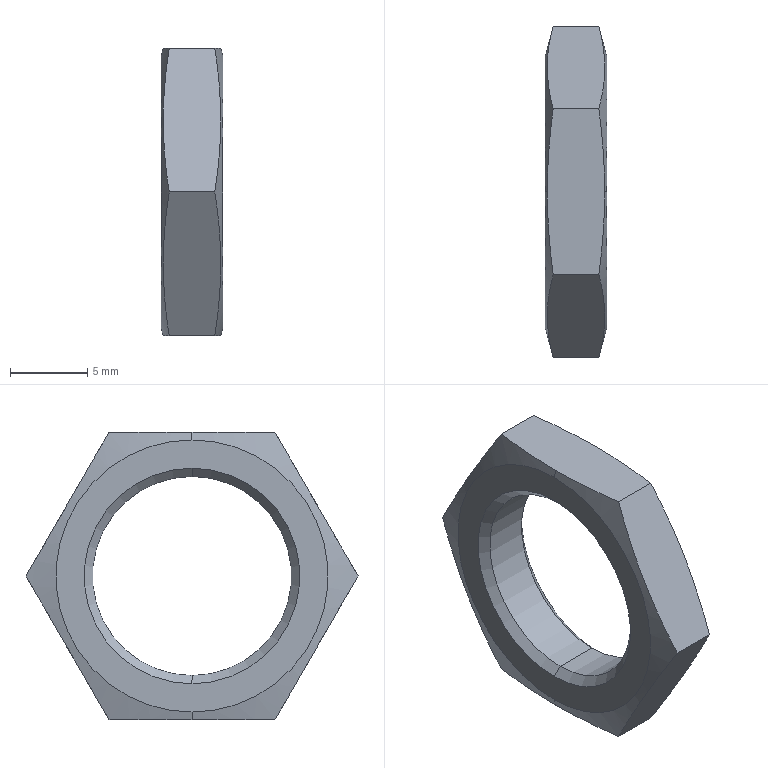Part | SolidWorks | features BaseBody 1 | 1 solid | 18 faces | box 4 x 21.554 x 18.667 mm | volume 652.633 mm3 | cone 8 | plane 8 | cylinder 2 | commonest cylinder face diameters 12.917 x2
STEP:
#1=CARTESIAN_POINT('',(0.5415,0.,-6.459));
#2=VERTEX_POINT('',#1);
#3=CARTESIAN_POINT('',(0.5415,0.,6.458));
#4=VERTEX_POINT('',#3);
#5=CARTESIAN_POINT('',(0.5415,0.,0.));
#6=DIRECTION('',(-1.,0.,0.));
#7=DIRECTION('',(0.,0.,1.));
#8=AXIS2_PLACEMENT_3D('',#5,#6,#7);
#9=CIRCLE('',#8,6.458);
#10=EDGE_CURVE('',#2,#4,#9,.T.);
#11=ORIENTED_EDGE('',*,*,#10,.F.);
#12=CARTESIAN_POINT('',(0.,0.,-7.));
#13=VERTEX_POINT('',#12);
#14=CARTESIAN_POINT('',(0.,0.,-7.));
#15=DIRECTION('',(-0.7071,0.,-0.7071));
#16=VECTOR('',#15,1000.);
#17=LINE('',#14,#16);
#18=EDGE_CURVE('',#2,#13,#17,.T.);
#19=ORIENTED_EDGE('',*,*,#18,.T.);
#20=CARTESIAN_POINT('',(0.,0.,7.));
#21=VERTEX_POINT('',#20);
#22=CARTESIAN_POINT('',(0.,0.,0.));
#23=DIRECTION('',(1.,0.,0.));
#24=DIRECTION('',(0.,0.,1.));
#25=AXIS2_PLACEMENT_3D('',#22,#23,#24);
#26=CIRCLE('',#25,7.);
#27=EDGE_CURVE('',#21,#13,#26,.T.);
#28=ORIENTED_EDGE('',*,*,#27,.F.);
#29=CARTESIAN_POINT('',(0.,0.,7.));
#30=DIRECTION('',(-0.7071,0.,0.7071));
#31=VECTOR('',#30,1000.);
#32=LINE('',#29,#31);
#33=EDGE_CURVE('',#4,#21,#32,.T.);
#34=ORIENTED_EDGE('',*,*,#33,.F.);
#35=EDGE_LOOP('',(#11,#19,#28,#34));
#36=FACE_OUTER_BOUND('',#35,.T.);
#37=CARTESIAN_POINT('',(0.,0.,0.));
#38=DIRECTION('',(-1.,0.,0.));
#39=DIRECTION('',(0.,0.,1.));
#40=AXIS2_PLACEMENT_3D('',#37,#38,#39);
#41=CONICAL_SURFACE('',#40,7.,0.7854);
#42=ADVANCED_FACE('',(#36),#41,.F.);
#43=CARTESIAN_POINT('',(0.,0.,8.833));
#44=VERTEX_POINT('',#43);
#45=CARTESIAN_POINT('',(0.,0.,-8.833));
#46=VERTEX_POINT('',#45);
#47=CARTESIAN_POINT('',(0.,0.,0.));
#48=DIRECTION('',(-1.,0.,0.));
#49=DIRECTION('',(0.,0.,-1.));
#50=AXIS2_PLACEMENT_3D('',#47,#48,#49);
#51=CIRCLE('',#50,8.833);
#52=EDGE_CURVE('',#44,#46,#51,.T.);
#53=ORIENTED_EDGE('',*,*,#52,.F.);
#54=CARTESIAN_POINT('',(0.134,0.,9.333));
#55=VERTEX_POINT('',#54);
#56=CARTESIAN_POINT('',(0.524,0.,10.789));
#57=DIRECTION('',(0.2588,0.,0.9659));
#58=VECTOR('',#57,1000.);
#59=LINE('',#56,#58);
#60=EDGE_CURVE('',#44,#55,#59,.T.);
#61=ORIENTED_EDGE('',*,*,#60,.T.);
#62=CARTESIAN_POINT('',(0.5209,5.389,9.333));
#63=VERTEX_POINT('',#62);
#64=CARTESIAN_POINT('',(0.134,0.,9.333));
#65=CARTESIAN_POINT('',(0.134,1.805,9.333));
#66=CARTESIAN_POINT('',(0.2813,3.6,9.333));
#67=CARTESIAN_POINT('',(0.5209,5.389,9.333));
#68=B_SPLINE_CURVE_WITH_KNOTS('',3,(#64,#65,#66,#67),.UNSPECIFIED.,.F.,.F.,(4,4),(0.,0.005402),.UNSPECIFIED.);
#69=EDGE_CURVE('',#55,#63,#68,.T.);
#70=ORIENTED_EDGE('',*,*,#69,.T.);
#71=CARTESIAN_POINT('',(0.5209,10.777,0.000000009));
#72=VERTEX_POINT('',#71);
#73=CARTESIAN_POINT('',(0.5209,5.389,9.333));
#74=CARTESIAN_POINT('',(0.4005,5.838,8.556));
#75=CARTESIAN_POINT('',(0.3028,6.287,7.778));
#76=CARTESIAN_POINT('',(0.1693,7.185,6.222));
#77=CARTESIAN_POINT('',(0.0986,8.083,4.667));
#78=CARTESIAN_POINT('',(0.1693,8.981,3.111));
#79=CARTESIAN_POINT('',(0.3028,9.879,1.556));
#80=CARTESIAN_POINT('',(0.4005,10.328,0.7778));
#81=CARTESIAN_POINT('',(0.5209,10.777,0.000000009));
#82=B_SPLINE_CURVE_WITH_KNOTS('',3,(#73,#74,#75,#76,#77,#78,#79,#80,#81),.UNSPECIFIED.,.F.,.F.,(4,2,1,2,4),(0.,0.002694,0.005389,0.008083,0.01078),.UNSPECIFIED.);
#83=EDGE_CURVE('',#63,#72,#82,.T.);
#84=ORIENTED_EDGE('',*,*,#83,.T.);
#85=CARTESIAN_POINT('',(0.5209,5.389,-9.333));
#86=VERTEX_POINT('',#85);
#87=CARTESIAN_POINT('',(0.5209,10.777,0.000000009));
#88=CARTESIAN_POINT('',(0.4005,10.328,-0.7778));
#89=CARTESIAN_POINT('',(0.3028,9.879,-1.556));
#90=CARTESIAN_POINT('',(0.1693,8.981,-3.111));
#91=CARTESIAN_POINT('',(0.0986,8.083,-4.667));
#92=CARTESIAN_POINT('',(0.1693,7.185,-6.222));
#93=CARTESIAN_POINT('',(0.3028,6.287,-7.778));
#94=CARTESIAN_POINT('',(0.4005,5.838,-8.556));
#95=CARTESIAN_POINT('',(0.5209,5.389,-9.333));
#96=B_SPLINE_CURVE_WITH_KNOTS('',3,(#87,#88,#89,#90,#91,#92,#93,#94,#95),.UNSPECIFIED.,.F.,.F.,(4,2,1,2,4),(0.,0.002694,0.005389,0.008083,0.01078),.UNSPECIFIED.);
#97=EDGE_CURVE('',#72,#86,#96,.T.);
#98=ORIENTED_EDGE('',*,*,#97,.T.);
#99=CARTESIAN_POINT('',(0.134,0.,-9.333));
#100=VERTEX_POINT('',#99);
#101=CARTESIAN_POINT('',(0.5209,5.389,-9.333));
#102=CARTESIAN_POINT('',(0.2813,3.6,-9.333));
#103=CARTESIAN_POINT('',(0.134,1.805,-9.333));
#104=CARTESIAN_POINT('',(0.134,0.,-9.333));
#105=B_SPLINE_CURVE_WITH_KNOTS('',3,(#101,#102,#103,#104),.UNSPECIFIED.,.F.,.F.,(4,4),(0.,0.005402),.UNSPECIFIED.);
#106=EDGE_CURVE('',#86,#100,#105,.T.);
#107=ORIENTED_EDGE('',*,*,#106,.T.);
#108=CARTESIAN_POINT('',(0.524,0.,-10.789));
#109=DIRECTION('',(0.2588,0.,-0.9659));
#110=VECTOR('',#109,1000.);
#111=LINE('',#108,#110);
#112=EDGE_CURVE('',#46,#100,#111,.T.);
#113=ORIENTED_EDGE('',*,*,#112,.F.);
#114=EDGE_LOOP('',(#53,#61,#70,#84,#98,#107,#113));
#115=FACE_OUTER_BOUND('',#114,.T.);
#116=CARTESIAN_POINT('',(0.524,0.,0.));
#117=DIRECTION('',(1.,0.,0.));
#118=DIRECTION('',(0.,0.,-1.));
#119=AXIS2_PLACEMENT_3D('',#116,#117,#118);
#120=CONICAL_SURFACE('',#119,10.789,1.309);
#121=ADVANCED_FACE('',(#115),#120,.T.);
#122=CARTESIAN_POINT('',(3.458,0.,-6.458));
#123=VERTEX_POINT('',#122);
#124=CARTESIAN_POINT('',(3.458,0.,6.458));
#125=VERTEX_POINT('',#124);
#126=CARTESIAN_POINT('',(3.458,0.,0.));
#127=DIRECTION('',(-1.,0.,0.));
#128=DIRECTION('',(0.,0.,1.));
#129=AXIS2_PLACEMENT_3D('',#126,#127,#128);
#130=CIRCLE('',#129,6.458);
#131=EDGE_CURVE('',#123,#125,#130,.T.);
#132=ORIENTED_EDGE('',*,*,#131,.F.);
#133=CARTESIAN_POINT('',(4.,0.,-6.458));
#134=DIRECTION('',(-1.,0.,0.));
#135=VECTOR('',#134,1000.);
#136=LINE('',#133,#135);
#137=EDGE_CURVE('',#123,#2,#136,.T.);
#138=ORIENTED_EDGE('',*,*,#137,.T.);
#139=ORIENTED_EDGE('',*,*,#10,.T.);
#140=CARTESIAN_POINT('',(4.,0.,6.458));
#141=DIRECTION('',(-1.,0.,0.));
#142=VECTOR('',#141,1000.);
#143=LINE('',#140,#142);
#144=EDGE_CURVE('',#125,#4,#143,.T.);
#145=ORIENTED_EDGE('',*,*,#144,.F.);
#146=EDGE_LOOP('',(#132,#138,#139,#145));
#147=FACE_OUTER_BOUND('',#146,.T.);
#148=CARTESIAN_POINT('',(4.,0.,0.));
#149=DIRECTION('',(-1.,0.,0.));
#150=DIRECTION('',(0.,0.,1.));
#151=AXIS2_PLACEMENT_3D('',#148,#149,#150);
#152=CYLINDRICAL_SURFACE('',#151,6.458);
#153=ADVANCED_FACE('',(#147),#152,.F.);
#154=ORIENTED_EDGE('',*,*,#131,.T.);
#155=CARTESIAN_POINT('',(4.,0.,7.));
#156=VERTEX_POINT('',#155);
#157=CARTESIAN_POINT('',(4.,0.,7.));
#158=DIRECTION('',(0.7071,0.,0.7071));
#159=VECTOR('',#158,1000.);
#160=LINE('',#157,#159);
#161=EDGE_CURVE('',#125,#156,#160,.T.);
#162=ORIENTED_EDGE('',*,*,#161,.T.);
#163=CARTESIAN_POINT('',(4.,0.,-7.));
#164=VERTEX_POINT('',#163);
#165=CARTESIAN_POINT('',(4.,0.,0.));
#166=DIRECTION('',(-1.,0.,0.));
#167=DIRECTION('',(0.,0.,-1.));
#168=AXIS2_PLACEMENT_3D('',#165,#166,#167);
#169=CIRCLE('',#168,7.);
#170=EDGE_CURVE('',#164,#156,#169,.T.);
#171=ORIENTED_EDGE('',*,*,#170,.F.);
#172=CARTESIAN_POINT('',(4.,0.,-7.));
#173=DIRECTION('',(0.7071,0.,-0.7071));
#174=VECTOR('',#173,1000.);
#175=LINE('',#172,#174);
#176=EDGE_CURVE('',#123,#164,#175,.T.);
#177=ORIENTED_EDGE('',*,*,#176,.F.);
#178=EDGE_LOOP('',(#154,#162,#171,#177));
#179=FACE_OUTER_BOUND('',#178,.T.);
#180=CARTESIAN_POINT('',(4.,0.,0.));
#181=DIRECTION('',(1.,0.,0.));
#182=DIRECTION('',(0.,0.,-1.));
#183=AXIS2_PLACEMENT_3D('',#180,#181,#182);
#184=CONICAL_SURFACE('',#183,7.,0.7854);
#185=ADVANCED_FACE('',(#179),#184,.F.);
#186=CARTESIAN_POINT('',(4.,0.,8.833));
#187=VERTEX_POINT('',#186);
#188=CARTESIAN_POINT('',(4.,0.,-8.833));
#189=VERTEX_POINT('',#188);
#190=CARTESIAN_POINT('',(4.,0.,0.));
#191=DIRECTION('',(-1.,0.,0.));
#192=DIRECTION('',(0.,0.,1.));
#193=AXIS2_PLACEMENT_3D('',#190,#191,#192);
#194=CIRCLE('',#193,8.833);
#195=EDGE_CURVE('',#187,#189,#194,.T.);
#196=ORIENTED_EDGE('',*,*,#195,.T.);
#197=CARTESIAN_POINT('',(3.866,0.,-9.333));
#198=VERTEX_POINT('',#197);
#199=CARTESIAN_POINT('',(3.476,0.,-10.789));
#200=DIRECTION('',(-0.2588,0.,-0.9659));
#201=VECTOR('',#200,1000.);
#202=LINE('',#199,#201);
#203=EDGE_CURVE('',#189,#198,#202,.T.);
#204=ORIENTED_EDGE('',*,*,#203,.T.);
#205=CARTESIAN_POINT('',(3.479,5.389,-9.333));
#206=VERTEX_POINT('',#205);
#207=CARTESIAN_POINT('',(3.866,0.,-9.333));
#208=CARTESIAN_POINT('',(3.866,1.805,-9.333));
#209=CARTESIAN_POINT('',(3.719,3.6,-9.333));
#210=CARTESIAN_POINT('',(3.479,5.389,-9.333));
#211=B_SPLINE_CURVE_WITH_KNOTS('',3,(#207,#208,#209,#210),.UNSPECIFIED.,.F.,.F.,(4,4),(0.,0.005402),.UNSPECIFIED.);
#212=EDGE_CURVE('',#198,#206,#211,.T.);
#213=ORIENTED_EDGE('',*,*,#212,.T.);
#214=CARTESIAN_POINT('',(3.479,10.777,-0.000000025));
#215=VERTEX_POINT('',#214);
#216=CARTESIAN_POINT('',(3.479,5.389,-9.333));
#217=CARTESIAN_POINT('',(3.599,5.838,-8.556));
#218=CARTESIAN_POINT('',(3.697,6.287,-7.778));
#219=CARTESIAN_POINT('',(3.831,7.185,-6.222));
#220=CARTESIAN_POINT('',(3.901,8.083,-4.667));
#221=CARTESIAN_POINT('',(3.831,8.981,-3.111));
#222=CARTESIAN_POINT('',(3.697,9.879,-1.556));
#223=CARTESIAN_POINT('',(3.599,10.328,-0.7778));
#224=CARTESIAN_POINT('',(3.479,10.777,-0.000000025));
#225=B_SPLINE_CURVE_WITH_KNOTS('',3,(#216,#217,#218,#219,#220,#221,#222,#223,#224),.UNSPECIFIED.,.F.,.F.,(4,2,1,2,4),(0.,0.002694,0.005389,0.008083,0.01078),.UNSPECIFIED.);
#226=EDGE_CURVE('',#206,#215,#225,.T.);
#227=ORIENTED_EDGE('',*,*,#226,.T.);
#228=CARTESIAN_POINT('',(3.479,5.389,9.333));
#229=VERTEX_POINT('',#228);
#230=CARTESIAN_POINT('',(3.479,10.777,-0.000000025));
#231=CARTESIAN_POINT('',(3.599,10.328,0.7778));
#232=CARTESIAN_POINT('',(3.697,9.879,1.556));
#233=CARTESIAN_POINT('',(3.831,8.981,3.111));
#234=CARTESIAN_POINT('',(3.901,8.083,4.667));
#235=CARTESIAN_POINT('',(3.831,7.185,6.222));
#236=CARTESIAN_POINT('',(3.697,6.287,7.778));
#237=CARTESIAN_POINT('',(3.599,5.838,8.556));
#238=CARTESIAN_POINT('',(3.479,5.389,9.333));
#239=B_SPLINE_CURVE_WITH_KNOTS('',3,(#230,#231,#232,#233,#234,#235,#236,#237,#238),.UNSPECIFIED.,.F.,.F.,(4,2,1,2,4),(0.,0.002694,0.005389,0.008083,0.01078),.UNSPECIFIED.);
#240=EDGE_CURVE('',#215,#229,#239,.T.);
#241=ORIENTED_EDGE('',*,*,#240,.T.);
#242=CARTESIAN_POINT('',(3.866,0.,9.333));
#243=VERTEX_POINT('',#242);
#244=CARTESIAN_POINT('',(3.479,5.389,9.333));
#245=CARTESIAN_POINT('',(3.719,3.6,9.333));
#246=CARTESIAN_POINT('',(3.866,1.805,9.333));
#247=CARTESIAN_POINT('',(3.866,0.,9.333));
#248=B_SPLINE_CURVE_WITH_KNOTS('',3,(#244,#245,#246,#247),.UNSPECIFIED.,.F.,.F.,(4,4),(-0.005402,0.),.UNSPECIFIED.);
#249=EDGE_CURVE('',#229,#243,#248,.T.);
#250=ORIENTED_EDGE('',*,*,#249,.T.);
#251=CARTESIAN_POINT('',(3.476,0.,10.789));
#252=DIRECTION('',(-0.2588,0.,0.9659));
#253=VECTOR('',#252,1000.);
#254=LINE('',#251,#253);
#255=EDGE_CURVE('',#187,#243,#254,.T.);
#256=ORIENTED_EDGE('',*,*,#255,.F.);
#257=EDGE_LOOP('',(#196,#204,#213,#227,#241,#250,#256));
#258=FACE_OUTER_BOUND('',#257,.T.);
#259=CARTESIAN_POINT('',(3.476,0.,0.));
#260=DIRECTION('',(-1.,0.,0.));
#261=DIRECTION('',(0.,0.,1.));
#262=AXIS2_PLACEMENT_3D('',#259,#260,#261);
#263=CONICAL_SURFACE('',#262,10.789,1.309);
#264=ADVANCED_FACE('',(#258),#263,.T.);
#265=ORIENTED_EDGE('',*,*,#27,.T.);
#266=CARTESIAN_POINT('',(0.,0.,0.));
#267=DIRECTION('',(1.,0.,0.));
#268=DIRECTION('',(0.,0.,1.));
#269=AXIS2_PLACEMENT_3D('',#266,#267,#268);
#270=CIRCLE('',#269,7.);
#271=EDGE_CURVE('',#13,#21,#270,.T.);
#272=ORIENTED_EDGE('',*,*,#271,.T.);
#273=EDGE_LOOP('',(#265,#272));
#274=FACE_BOUND('',#273,.T.);
#275=CARTESIAN_POINT('',(0.,0.,0.));
#276=DIRECTION('',(-1.,0.,0.));
#277=DIRECTION('',(0.,0.,-1.));
#278=AXIS2_PLACEMENT_3D('',#275,#276,#277);
#279=CIRCLE('',#278,8.833);
#280=EDGE_CURVE('',#46,#44,#279,.T.);
#281=ORIENTED_EDGE('',*,*,#280,.T.);
#282=ORIENTED_EDGE('',*,*,#52,.T.);
#283=EDGE_LOOP('',(#281,#282));
#284=FACE_OUTER_BOUND('',#283,.T.);
#285=CARTESIAN_POINT('',(0.,8.833,0.));
#286=DIRECTION('',(-1.,0.,0.));
#287=DIRECTION('',(0.,0.,1.));
#288=AXIS2_PLACEMENT_3D('',#285,#286,#287);
#289=PLANE('',#288);
#290=ADVANCED_FACE('',(#274,#284),#289,.T.);
#291=ORIENTED_EDGE('',*,*,#18,.F.);
#292=CARTESIAN_POINT('',(0.5415,0.,0.));
#293=DIRECTION('',(-1.,0.,0.));
#294=DIRECTION('',(0.,0.,1.));
#295=AXIS2_PLACEMENT_3D('',#292,#293,#294);
#296=CIRCLE('',#295,6.458);
#297=EDGE_CURVE('',#4,#2,#296,.T.);
#298=ORIENTED_EDGE('',*,*,#297,.F.);
#299=ORIENTED_EDGE('',*,*,#33,.T.);
#300=ORIENTED_EDGE('',*,*,#271,.F.);
#301=EDGE_LOOP('',(#291,#298,#299,#300));
#302=FACE_OUTER_BOUND('',#301,.T.);
#303=CARTESIAN_POINT('',(0.,0.,0.));
#304=DIRECTION('',(-1.,0.,0.));
#305=DIRECTION('',(0.,0.,1.));
#306=AXIS2_PLACEMENT_3D('',#303,#304,#305);
#307=CONICAL_SURFACE('',#306,7.,0.7854);
#308=ADVANCED_FACE('',(#302),#307,.F.);
#309=ORIENTED_EDGE('',*,*,#60,.F.);
#310=ORIENTED_EDGE('',*,*,#280,.F.);
#311=ORIENTED_EDGE('',*,*,#112,.T.);
#312=CARTESIAN_POINT('',(0.5209,-5.389,-9.333));
#313=VERTEX_POINT('',#312);
#314=CARTESIAN_POINT('',(0.134,0.,-9.333));
#315=CARTESIAN_POINT('',(0.134,-1.805,-9.333));
#316=CARTESIAN_POINT('',(0.2813,-3.6,-9.333));
#317=CARTESIAN_POINT('',(0.5209,-5.389,-9.333));
#318=B_SPLINE_CURVE_WITH_KNOTS('',3,(#314,#315,#316,#317),.UNSPECIFIED.,.F.,.F.,(4,4),(0.005402,0.0108),.UNSPECIFIED.);
#319=EDGE_CURVE('',#100,#313,#318,.T.);
#320=ORIENTED_EDGE('',*,*,#319,.T.);
#321=CARTESIAN_POINT('',(0.5209,-10.777,-0.000000009));
#322=VERTEX_POINT('',#321);
#323=CARTESIAN_POINT('',(0.5209,-5.389,-9.333));
#324=CARTESIAN_POINT('',(0.4005,-5.838,-8.556));
#325=CARTESIAN_POINT('',(0.3028,-6.287,-7.778));
#326=CARTESIAN_POINT('',(0.1693,-7.185,-6.222));
#327=CARTESIAN_POINT('',(0.0986,-8.083,-4.667));
#328=CARTESIAN_POINT('',(0.1693,-8.981,-3.111));
#329=CARTESIAN_POINT('',(0.3028,-9.879,-1.556));
#330=CARTESIAN_POINT('',(0.4005,-10.328,-0.7778));
#331=CARTESIAN_POINT('',(0.5209,-10.777,-0.000000009));
#332=B_SPLINE_CURVE_WITH_KNOTS('',3,(#323,#324,#325,#326,#327,#328,#329,#330,#331),.UNSPECIFIED.,.F.,.F.,(4,2,1,2,4),(0.,0.002694,0.005389,0.008083,0.01078),.UNSPECIFIED.);
#333=EDGE_CURVE('',#313,#322,#332,.T.);
#334=ORIENTED_EDGE('',*,*,#333,.T.);
#335=CARTESIAN_POINT('',(0.5209,-5.389,9.333));
#336=VERTEX_POINT('',#335);
#337=CARTESIAN_POINT('',(0.5209,-10.777,-0.000000009));
#338=CARTESIAN_POINT('',(0.4005,-10.328,0.7778));
#339=CARTESIAN_POINT('',(0.3028,-9.879,1.556));
#340=CARTESIAN_POINT('',(0.1693,-8.981,3.111));
#341=CARTESIAN_POINT('',(0.0986,-8.083,4.667));
#342=CARTESIAN_POINT('',(0.1693,-7.185,6.222));
#343=CARTESIAN_POINT('',(0.3028,-6.287,7.778));
#344=CARTESIAN_POINT('',(0.4005,-5.838,8.556));
#345=CARTESIAN_POINT('',(0.5209,-5.389,9.333));
#346=B_SPLINE_CURVE_WITH_KNOTS('',3,(#337,#338,#339,#340,#341,#342,#343,#344,#345),.UNSPECIFIED.,.F.,.F.,(4,2,1,2,4),(0.,0.002694,0.005389,0.008083,0.01078),.UNSPECIFIED.);
#347=EDGE_CURVE('',#322,#336,#346,.T.);
#348=ORIENTED_EDGE('',*,*,#347,.T.);
#349=CARTESIAN_POINT('',(0.5209,-5.389,9.333));
#350=CARTESIAN_POINT('',(0.2813,-3.6,9.333));
#351=CARTESIAN_POINT('',(0.134,-1.805,9.333));
#352=CARTESIAN_POINT('',(0.134,0.,9.333));
#353=B_SPLINE_CURVE_WITH_KNOTS('',3,(#349,#350,#351,#352),.UNSPECIFIED.,.F.,.F.,(4,4),(-0.005402,0.),.UNSPECIFIED.);
#354=EDGE_CURVE('',#336,#55,#353,.T.);
#355=ORIENTED_EDGE('',*,*,#354,.T.);
#356=EDGE_LOOP('',(#309,#310,#311,#320,#334,#348,#355));
#357=FACE_OUTER_BOUND('',#356,.T.);
#358=CARTESIAN_POINT('',(0.524,0.,0.));
#359=DIRECTION('',(1.,0.,0.));
#360=DIRECTION('',(0.,0.,-1.));
#361=AXIS2_PLACEMENT_3D('',#358,#359,#360);
#362=CONICAL_SURFACE('',#361,10.789,1.309);
#363=ADVANCED_FACE('',(#357),#362,.T.);
#364=ORIENTED_EDGE('',*,*,#137,.F.);
#365=CARTESIAN_POINT('',(3.458,0.,0.));
#366=DIRECTION('',(-1.,0.,0.));
#367=DIRECTION('',(0.,0.,1.));
#368=AXIS2_PLACEMENT_3D('',#365,#366,#367);
#369=CIRCLE('',#368,6.458);
#370=EDGE_CURVE('',#125,#123,#369,.T.);
#371=ORIENTED_EDGE('',*,*,#370,.F.);
#372=ORIENTED_EDGE('',*,*,#144,.T.);
#373=ORIENTED_EDGE('',*,*,#297,.T.);
#374=EDGE_LOOP('',(#364,#371,#372,#373));
#375=FACE_OUTER_BOUND('',#374,.T.);
#376=CARTESIAN_POINT('',(4.,0.,0.));
#377=DIRECTION('',(-1.,0.,0.));
#378=DIRECTION('',(0.,0.,1.));
#379=AXIS2_PLACEMENT_3D('',#376,#377,#378);
#380=CYLINDRICAL_SURFACE('',#379,6.458);
#381=ADVANCED_FACE('',(#375),#380,.F.);
#382=CARTESIAN_POINT('',(3.479,-5.389,-9.333));
#383=VERTEX_POINT('',#382);
#384=CARTESIAN_POINT('',(4.,-5.389,-9.333));
#385=DIRECTION('',(1.,0.,0.));
#386=VECTOR('',#385,1000.);
#387=LINE('',#384,#386);
#388=EDGE_CURVE('',#313,#383,#387,.T.);
#389=ORIENTED_EDGE('',*,*,#388,.F.);
#390=ORIENTED_EDGE('',*,*,#319,.F.);
#391=ORIENTED_EDGE('',*,*,#106,.F.);
#392=CARTESIAN_POINT('',(4.,5.389,-9.333));
#393=DIRECTION('',(-1.,0.,0.));
#394=VECTOR('',#393,1000.);
#395=LINE('',#392,#394);
#396=EDGE_CURVE('',#206,#86,#395,.T.);
#397=ORIENTED_EDGE('',*,*,#396,.F.);
#398=ORIENTED_EDGE('',*,*,#212,.F.);
#399=CARTESIAN_POINT('',(3.479,-5.389,-9.333));
#400=CARTESIAN_POINT('',(3.719,-3.6,-9.333));
#401=CARTESIAN_POINT('',(3.866,-1.805,-9.333));
#402=CARTESIAN_POINT('',(3.866,0.,-9.333));
#403=B_SPLINE_CURVE_WITH_KNOTS('',3,(#399,#400,#401,#402),.UNSPECIFIED.,.F.,.F.,(4,4),(-0.005402,0.),.UNSPECIFIED.);
#404=EDGE_CURVE('',#383,#198,#403,.T.);
#405=ORIENTED_EDGE('',*,*,#404,.F.);
#406=EDGE_LOOP('',(#389,#390,#391,#397,#398,#405));
#407=FACE_OUTER_BOUND('',#406,.T.);
#408=CARTESIAN_POINT('',(4.,-5.389,-9.333));
#409=DIRECTION('',(0.,0.,1.));
#410=DIRECTION('',(1.,0.,0.));
#411=AXIS2_PLACEMENT_3D('',#408,#409,#410);
#412=PLANE('',#411);
#413=ADVANCED_FACE('',(#407),#412,.F.);
#414=ORIENTED_EDGE('',*,*,#97,.F.);
#415=CARTESIAN_POINT('',(4.,10.777,-0.000000042));
#416=DIRECTION('',(-1.,0.,0.));
#417=VECTOR('',#416,1000.);
#418=LINE('',#415,#417);
#419=EDGE_CURVE('',#215,#72,#418,.T.);
#420=ORIENTED_EDGE('',*,*,#419,.F.);
#421=ORIENTED_EDGE('',*,*,#226,.F.);
#422=ORIENTED_EDGE('',*,*,#396,.T.);
#423=EDGE_LOOP('',(#414,#420,#421,#422));
#424=FACE_OUTER_BOUND('',#423,.T.);
#425=CARTESIAN_POINT('',(4.,5.389,-9.333));
#426=DIRECTION('',(0.,-0.866,0.5));
#427=DIRECTION('',(0.,-0.5,-0.866));
#428=AXIS2_PLACEMENT_3D('',#425,#426,#427);
#429=PLANE('',#428);
#430=ADVANCED_FACE('',(#424),#429,.F.);
#431=ORIENTED_EDGE('',*,*,#83,.F.);
#432=CARTESIAN_POINT('',(4.,5.389,9.333));
#433=DIRECTION('',(-1.,0.,0.));
#434=VECTOR('',#433,1000.);
#435=LINE('',#432,#434);
#436=EDGE_CURVE('',#229,#63,#435,.T.);
#437=ORIENTED_EDGE('',*,*,#436,.F.);
#438=ORIENTED_EDGE('',*,*,#240,.F.);
#439=ORIENTED_EDGE('',*,*,#419,.T.);
#440=EDGE_LOOP('',(#431,#437,#438,#439));
#441=FACE_OUTER_BOUND('',#440,.T.);
#442=CARTESIAN_POINT('',(4.,10.777,0.));
#443=DIRECTION('',(0.,-0.866,-0.5));
#444=DIRECTION('',(0.,0.5,-0.866));
#445=AXIS2_PLACEMENT_3D('',#442,#443,#444);
#446=PLANE('',#445);
#447=ADVANCED_FACE('',(#441),#446,.F.);
#448=ORIENTED_EDGE('',*,*,#354,.F.);
#449=CARTESIAN_POINT('',(3.479,-5.389,9.333));
#450=VERTEX_POINT('',#449);
#451=CARTESIAN_POINT('',(4.,-5.389,9.333));
#452=DIRECTION('',(-1.,0.,0.));
#453=VECTOR('',#452,1000.);
#454=LINE('',#451,#453);
#455=EDGE_CURVE('',#450,#336,#454,.T.);
#456=ORIENTED_EDGE('',*,*,#455,.F.);
#457=CARTESIAN_POINT('',(3.866,0.,9.333));
#458=CARTESIAN_POINT('',(3.866,-1.805,9.333));
#459=CARTESIAN_POINT('',(3.719,-3.6,9.333));
#460=CARTESIAN_POINT('',(3.479,-5.389,9.333));
#461=B_SPLINE_CURVE_WITH_KNOTS('',3,(#457,#458,#459,#460),.UNSPECIFIED.,.F.,.F.,(4,4),(0.,0.005402),.UNSPECIFIED.);
#462=EDGE_CURVE('',#243,#450,#461,.T.);
#463=ORIENTED_EDGE('',*,*,#462,.F.);
#464=ORIENTED_EDGE('',*,*,#249,.F.);
#465=ORIENTED_EDGE('',*,*,#436,.T.);
#466=ORIENTED_EDGE('',*,*,#69,.F.);
#467=EDGE_LOOP('',(#448,#456,#463,#464,#465,#466));
#468=FACE_OUTER_BOUND('',#467,.T.);
#469=CARTESIAN_POINT('',(4.,5.389,9.333));
#470=DIRECTION('',(0.,0.,-1.));
#471=DIRECTION('',(-1.,0.,0.));
#472=AXIS2_PLACEMENT_3D('',#469,#470,#471);
#473=PLANE('',#472);
#474=ADVANCED_FACE('',(#468),#473,.F.);
#475=ORIENTED_EDGE('',*,*,#347,.F.);
#476=CARTESIAN_POINT('',(3.479,-10.777,0.000000015));
#477=VERTEX_POINT('',#476);
#478=CARTESIAN_POINT('',(4.,-10.777,0.000000042));
#479=DIRECTION('',(-1.,0.,0.));
#480=VECTOR('',#479,1000.);
#481=LINE('',#478,#480);
#482=EDGE_CURVE('',#477,#322,#481,.T.);
#483=ORIENTED_EDGE('',*,*,#482,.F.);
#484=CARTESIAN_POINT('',(3.479,-5.389,9.333));
#485=CARTESIAN_POINT('',(3.599,-5.838,8.556));
#486=CARTESIAN_POINT('',(3.697,-6.287,7.778));
#487=CARTESIAN_POINT('',(3.831,-7.185,6.222));
#488=CARTESIAN_POINT('',(3.901,-8.083,4.667));
#489=CARTESIAN_POINT('',(3.831,-8.981,3.111));
#490=CARTESIAN_POINT('',(3.697,-9.879,1.556));
#491=CARTESIAN_POINT('',(3.599,-10.328,0.7778));
#492=CARTESIAN_POINT('',(3.479,-10.777,0.000000015));
#493=B_SPLINE_CURVE_WITH_KNOTS('',3,(#484,#485,#486,#487,#488,#489,#490,#491,#492),.UNSPECIFIED.,.F.,.F.,(4,2,1,2,4),(0.,0.002694,0.005389,0.008083,0.01078),.UNSPECIFIED.);
#494=EDGE_CURVE('',#450,#477,#493,.T.);
#495=ORIENTED_EDGE('',*,*,#494,.F.);
#496=ORIENTED_EDGE('',*,*,#455,.T.);
#497=EDGE_LOOP('',(#475,#483,#495,#496));
#498=FACE_OUTER_BOUND('',#497,.T.);
#499=CARTESIAN_POINT('',(4.,-5.389,9.333));
#500=DIRECTION('',(0.,0.866,-0.5));
#501=DIRECTION('',(0.,0.5,0.866));
#502=AXIS2_PLACEMENT_3D('',#499,#500,#501);
#503=PLANE('',#502);
#504=ADVANCED_FACE('',(#498),#503,.F.);
#505=ORIENTED_EDGE('',*,*,#333,.F.);
#506=ORIENTED_EDGE('',*,*,#388,.T.);
#507=CARTESIAN_POINT('',(3.479,-10.777,0.000000015));
#508=CARTESIAN_POINT('',(3.599,-10.328,-0.7778));
#509=CARTESIAN_POINT('',(3.697,-9.879,-1.556));
#510=CARTESIAN_POINT('',(3.831,-8.981,-3.111));
#511=CARTESIAN_POINT('',(3.901,-8.083,-4.667));
#512=CARTESIAN_POINT('',(3.831,-7.185,-6.222));
#513=CARTESIAN_POINT('',(3.697,-6.287,-7.778));
#514=CARTESIAN_POINT('',(3.599,-5.838,-8.556));
#515=CARTESIAN_POINT('',(3.479,-5.389,-9.333));
#516=B_SPLINE_CURVE_WITH_KNOTS('',3,(#507,#508,#509,#510,#511,#512,#513,#514,#515),.UNSPECIFIED.,.F.,.F.,(4,2,1,2,4),(0.,0.002694,0.005389,0.008083,0.01078),.UNSPECIFIED.);
#517=EDGE_CURVE('',#477,#383,#516,.T.);
#518=ORIENTED_EDGE('',*,*,#517,.F.);
#519=ORIENTED_EDGE('',*,*,#482,.T.);
#520=EDGE_LOOP('',(#505,#506,#518,#519));
#521=FACE_OUTER_BOUND('',#520,.T.);
#522=CARTESIAN_POINT('',(4.,-10.777,0.));
#523=DIRECTION('',(0.,0.866,0.5));
#524=DIRECTION('',(0.,-0.5,0.866));
#525=AXIS2_PLACEMENT_3D('',#522,#523,#524);
#526=PLANE('',#525);
#527=ADVANCED_FACE('',(#521),#526,.F.);
#528=ORIENTED_EDGE('',*,*,#161,.F.);
#529=ORIENTED_EDGE('',*,*,#370,.T.);
#530=ORIENTED_EDGE('',*,*,#176,.T.);
#531=CARTESIAN_POINT('',(4.,0.,0.));
#532=DIRECTION('',(-1.,0.,0.));
#533=DIRECTION('',(0.,0.,-1.));
#534=AXIS2_PLACEMENT_3D('',#531,#532,#533);
#535=CIRCLE('',#534,7.);
#536=EDGE_CURVE('',#156,#164,#535,.T.);
#537=ORIENTED_EDGE('',*,*,#536,.F.);
#538=EDGE_LOOP('',(#528,#529,#530,#537));
#539=FACE_OUTER_BOUND('',#538,.T.);
#540=CARTESIAN_POINT('',(4.,0.,0.));
#541=DIRECTION('',(1.,0.,0.));
#542=DIRECTION('',(0.,0.,-1.));
#543=AXIS2_PLACEMENT_3D('',#540,#541,#542);
#544=CONICAL_SURFACE('',#543,7.,0.7854);
#545=ADVANCED_FACE('',(#539),#544,.F.);
#546=ORIENTED_EDGE('',*,*,#203,.F.);
#547=CARTESIAN_POINT('',(4.,0.,0.));
#548=DIRECTION('',(-1.,0.,0.));
#549=DIRECTION('',(0.,0.,1.));
#550=AXIS2_PLACEMENT_3D('',#547,#548,#549);
#551=CIRCLE('',#550,8.833);
#552=EDGE_CURVE('',#189,#187,#551,.T.);
#553=ORIENTED_EDGE('',*,*,#552,.T.);
#554=ORIENTED_EDGE('',*,*,#255,.T.);
#555=ORIENTED_EDGE('',*,*,#462,.T.);
#556=ORIENTED_EDGE('',*,*,#494,.T.);
#557=ORIENTED_EDGE('',*,*,#517,.T.);
#558=ORIENTED_EDGE('',*,*,#404,.T.);
#559=EDGE_LOOP('',(#546,#553,#554,#555,#556,#557,#558));
#560=FACE_OUTER_BOUND('',#559,.T.);
#561=CARTESIAN_POINT('',(3.476,0.,0.));
#562=DIRECTION('',(-1.,0.,0.));
#563=DIRECTION('',(0.,0.,1.));
#564=AXIS2_PLACEMENT_3D('',#561,#562,#563);
#565=CONICAL_SURFACE('',#564,10.789,1.309);
#566=ADVANCED_FACE('',(#560),#565,.T.);
#567=ORIENTED_EDGE('',*,*,#195,.F.);
#568=ORIENTED_EDGE('',*,*,#552,.F.);
#569=EDGE_LOOP('',(#567,#568));
#570=FACE_OUTER_BOUND('',#569,.T.);
#571=ORIENTED_EDGE('',*,*,#170,.T.);
#572=ORIENTED_EDGE('',*,*,#536,.T.);
#573=EDGE_LOOP('',(#571,#572));
#574=FACE_BOUND('',#573,.T.);
#575=CARTESIAN_POINT('',(4.,7.,0.));
#576=DIRECTION('',(1.,0.,0.));
#577=DIRECTION('',(0.,0.,-1.));
#578=AXIS2_PLACEMENT_3D('',#575,#576,#577);
#579=PLANE('',#578);
#580=ADVANCED_FACE('',(#570,#574),#579,.T.);
#581=CLOSED_SHELL('',(#42,#121,#153,#185,#264,#290,#308,#363,#381,#413,#430,#447,#474,#504,#527,#545,#566,#580));
#582=MANIFOLD_SOLID_BREP('',#581);
#583=CARTESIAN_POINT('',(0.,0.,0.));
#584=DIRECTION('',(0.,0.,1.));
#585=DIRECTION('',(1.,0.,0.));
#586=AXIS2_PLACEMENT_3D('',#583,#584,#585);
#587=(LENGTH_UNIT()NAMED_UNIT(*)SI_UNIT(.MILLI.,.METRE.));
#588=UNCERTAINTY_MEASURE_WITH_UNIT(LENGTH_MEASURE(0.00001),#587,'','');
#589=(NAMED_UNIT(*)PLANE_ANGLE_UNIT()SI_UNIT($,.RADIAN.));
#590=(NAMED_UNIT(*)SI_UNIT($,.STERADIAN.)SOLID_ANGLE_UNIT());
#591=(GEOMETRIC_REPRESENTATION_CONTEXT(3)GLOBAL_UNCERTAINTY_ASSIGNED_CONTEXT((#588))GLOBAL_UNIT_ASSIGNED_CONTEXT((#587,#589,#590))REPRESENTATION_CONTEXT('',''));
#592=ADVANCED_BREP_SHAPE_REPRESENTATION('',(#582,#586),#591);